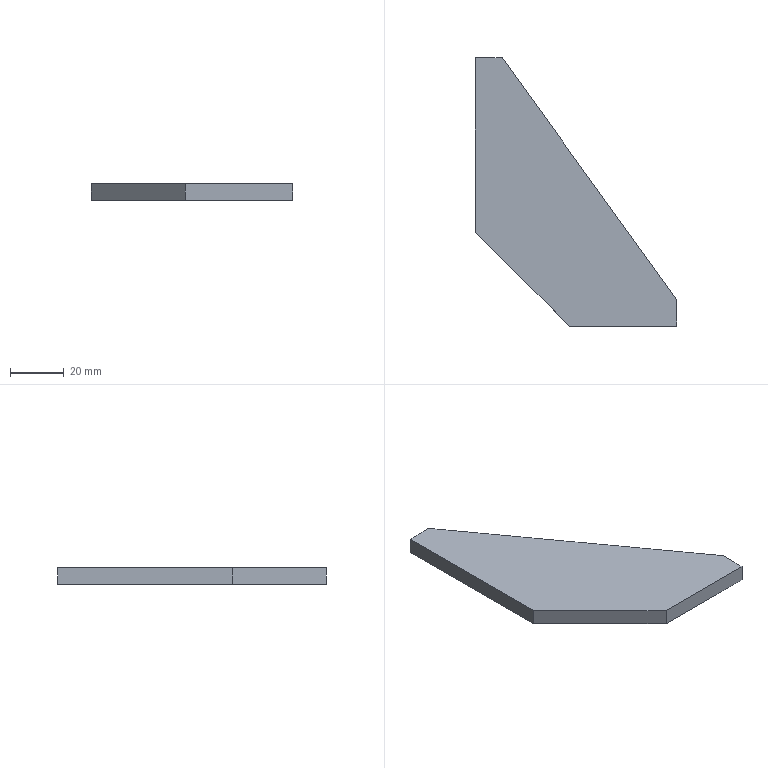Part | SolidWorks | features Chamfer 1, Extrusion 1 | 1 solid | 8 faces | box 75 x 100 x 6 mm | volume 23775 mm3 | plane 8
STEP:
#1=CARTESIAN_POINT('',(10.,100.,-3.));
#2=VERTEX_POINT('',#1);
#3=CARTESIAN_POINT('',(0.,100.,-3.));
#4=VERTEX_POINT('',#3);
#5=CARTESIAN_POINT('',(10.,100.,-3.));
#6=DIRECTION('',(-1.,0.,0.));
#7=VECTOR('',#6,1000.);
#8=LINE('',#5,#7);
#9=EDGE_CURVE('',#2,#4,#8,.T.);
#10=ORIENTED_EDGE('',*,*,#9,.T.);
#11=CARTESIAN_POINT('',(0.,100.,3.));
#12=VERTEX_POINT('',#11);
#13=CARTESIAN_POINT('',(0.,100.,3.));
#14=DIRECTION('',(0.,0.,-1.));
#15=VECTOR('',#14,1000.);
#16=LINE('',#13,#15);
#17=EDGE_CURVE('',#12,#4,#16,.T.);
#18=ORIENTED_EDGE('',*,*,#17,.F.);
#19=CARTESIAN_POINT('',(10.,100.,3.));
#20=VERTEX_POINT('',#19);
#21=CARTESIAN_POINT('',(10.,100.,3.));
#22=DIRECTION('',(-1.,0.,0.));
#23=VECTOR('',#22,1000.);
#24=LINE('',#21,#23);
#25=EDGE_CURVE('',#20,#12,#24,.T.);
#26=ORIENTED_EDGE('',*,*,#25,.F.);
#27=CARTESIAN_POINT('',(10.,100.,3.));
#28=DIRECTION('',(0.,0.,-1.));
#29=VECTOR('',#28,1000.);
#30=LINE('',#27,#29);
#31=EDGE_CURVE('',#20,#2,#30,.T.);
#32=ORIENTED_EDGE('',*,*,#31,.T.);
#33=EDGE_LOOP('',(#10,#18,#26,#32));
#34=FACE_OUTER_BOUND('',#33,.T.);
#35=CARTESIAN_POINT('',(10.,100.,3.));
#36=DIRECTION('',(0.,-1.,0.));
#37=DIRECTION('',(0.,0.,-1.));
#38=AXIS2_PLACEMENT_3D('',#35,#36,#37);
#39=PLANE('',#38);
#40=ADVANCED_FACE('',(#34),#39,.F.);
#41=CARTESIAN_POINT('',(0.,35.,-3.));
#42=VERTEX_POINT('',#41);
#43=CARTESIAN_POINT('',(0.,100.,-3.));
#44=DIRECTION('',(0.,-1.,0.));
#45=VECTOR('',#44,1000.);
#46=LINE('',#43,#45);
#47=EDGE_CURVE('',#4,#42,#46,.T.);
#48=ORIENTED_EDGE('',*,*,#47,.T.);
#49=CARTESIAN_POINT('',(0.,35.,3.));
#50=VERTEX_POINT('',#49);
#51=CARTESIAN_POINT('',(0.,35.,3.));
#52=DIRECTION('',(0.,0.,1.));
#53=VECTOR('',#52,1000.);
#54=LINE('',#51,#53);
#55=EDGE_CURVE('',#42,#50,#54,.T.);
#56=ORIENTED_EDGE('',*,*,#55,.T.);
#57=CARTESIAN_POINT('',(0.,100.,3.));
#58=DIRECTION('',(0.,-1.,0.));
#59=VECTOR('',#58,1000.);
#60=LINE('',#57,#59);
#61=EDGE_CURVE('',#12,#50,#60,.T.);
#62=ORIENTED_EDGE('',*,*,#61,.F.);
#63=ORIENTED_EDGE('',*,*,#17,.T.);
#64=EDGE_LOOP('',(#48,#56,#62,#63));
#65=FACE_OUTER_BOUND('',#64,.T.);
#66=CARTESIAN_POINT('',(0.,100.,3.));
#67=DIRECTION('',(1.,0.,0.));
#68=DIRECTION('',(0.,1.,0.));
#69=AXIS2_PLACEMENT_3D('',#66,#67,#68);
#70=PLANE('',#69);
#71=ADVANCED_FACE('',(#65),#70,.F.);
#72=CARTESIAN_POINT('',(35.,0.,3.));
#73=VERTEX_POINT('',#72);
#74=CARTESIAN_POINT('',(75.,0.,3.));
#75=VERTEX_POINT('',#74);
#76=CARTESIAN_POINT('',(0.,0.,3.));
#77=DIRECTION('',(1.,0.,0.));
#78=VECTOR('',#77,1000.);
#79=LINE('',#76,#78);
#80=EDGE_CURVE('',#73,#75,#79,.T.);
#81=ORIENTED_EDGE('',*,*,#80,.F.);
#82=CARTESIAN_POINT('',(35.,0.,-3.));
#83=VERTEX_POINT('',#82);
#84=CARTESIAN_POINT('',(35.,0.,3.));
#85=DIRECTION('',(0.,0.,-1.));
#86=VECTOR('',#85,1000.);
#87=LINE('',#84,#86);
#88=EDGE_CURVE('',#73,#83,#87,.T.);
#89=ORIENTED_EDGE('',*,*,#88,.T.);
#90=CARTESIAN_POINT('',(75.,0.,-3.));
#91=VERTEX_POINT('',#90);
#92=CARTESIAN_POINT('',(0.,0.,-3.));
#93=DIRECTION('',(1.,0.,0.));
#94=VECTOR('',#93,1000.);
#95=LINE('',#92,#94);
#96=EDGE_CURVE('',#83,#91,#95,.T.);
#97=ORIENTED_EDGE('',*,*,#96,.T.);
#98=CARTESIAN_POINT('',(75.,0.,3.));
#99=DIRECTION('',(0.,0.,-1.));
#100=VECTOR('',#99,1000.);
#101=LINE('',#98,#100);
#102=EDGE_CURVE('',#75,#91,#101,.T.);
#103=ORIENTED_EDGE('',*,*,#102,.F.);
#104=EDGE_LOOP('',(#81,#89,#97,#103));
#105=FACE_OUTER_BOUND('',#104,.T.);
#106=CARTESIAN_POINT('',(0.,0.,3.));
#107=DIRECTION('',(0.,1.,0.));
#108=DIRECTION('',(0.,0.,1.));
#109=AXIS2_PLACEMENT_3D('',#106,#107,#108);
#110=PLANE('',#109);
#111=ADVANCED_FACE('',(#105),#110,.F.);
#112=CARTESIAN_POINT('',(75.,10.,-3.));
#113=VERTEX_POINT('',#112);
#114=CARTESIAN_POINT('',(75.,0.,-3.));
#115=DIRECTION('',(0.,1.,0.));
#116=VECTOR('',#115,1000.);
#117=LINE('',#114,#116);
#118=EDGE_CURVE('',#91,#113,#117,.T.);
#119=ORIENTED_EDGE('',*,*,#118,.T.);
#120=CARTESIAN_POINT('',(75.,10.,3.));
#121=VERTEX_POINT('',#120);
#122=CARTESIAN_POINT('',(75.,10.,3.));
#123=DIRECTION('',(0.,0.,-1.));
#124=VECTOR('',#123,1000.);
#125=LINE('',#122,#124);
#126=EDGE_CURVE('',#121,#113,#125,.T.);
#127=ORIENTED_EDGE('',*,*,#126,.F.);
#128=CARTESIAN_POINT('',(75.,0.,3.));
#129=DIRECTION('',(0.,1.,0.));
#130=VECTOR('',#129,1000.);
#131=LINE('',#128,#130);
#132=EDGE_CURVE('',#75,#121,#131,.T.);
#133=ORIENTED_EDGE('',*,*,#132,.F.);
#134=ORIENTED_EDGE('',*,*,#102,.T.);
#135=EDGE_LOOP('',(#119,#127,#133,#134));
#136=FACE_OUTER_BOUND('',#135,.T.);
#137=CARTESIAN_POINT('',(75.,0.,3.));
#138=DIRECTION('',(-1.,0.,0.));
#139=DIRECTION('',(0.,0.,1.));
#140=AXIS2_PLACEMENT_3D('',#137,#138,#139);
#141=PLANE('',#140);
#142=ADVANCED_FACE('',(#136),#141,.F.);
#143=CARTESIAN_POINT('',(75.,10.,-3.));
#144=DIRECTION('',(-0.5855,0.8107,0.));
#145=VECTOR('',#144,1000.);
#146=LINE('',#143,#145);
#147=EDGE_CURVE('',#113,#2,#146,.T.);
#148=ORIENTED_EDGE('',*,*,#147,.T.);
#149=ORIENTED_EDGE('',*,*,#31,.F.);
#150=CARTESIAN_POINT('',(75.,10.,3.));
#151=DIRECTION('',(-0.5855,0.8107,0.));
#152=VECTOR('',#151,1000.);
#153=LINE('',#150,#152);
#154=EDGE_CURVE('',#121,#20,#153,.T.);
#155=ORIENTED_EDGE('',*,*,#154,.F.);
#156=ORIENTED_EDGE('',*,*,#126,.T.);
#157=EDGE_LOOP('',(#148,#149,#155,#156));
#158=FACE_OUTER_BOUND('',#157,.T.);
#159=CARTESIAN_POINT('',(75.,10.,3.));
#160=DIRECTION('',(-0.8107,-0.5855,0.));
#161=DIRECTION('',(0.5855,-0.8107,0.));
#162=AXIS2_PLACEMENT_3D('',#159,#160,#161);
#163=PLANE('',#162);
#164=ADVANCED_FACE('',(#158),#163,.F.);
#165=ORIENTED_EDGE('',*,*,#61,.T.);
#166=CARTESIAN_POINT('',(17.5,17.5,3.));
#167=DIRECTION('',(0.7071,-0.7071,0.));
#168=VECTOR('',#167,1000.);
#169=LINE('',#166,#168);
#170=EDGE_CURVE('',#50,#73,#169,.T.);
#171=ORIENTED_EDGE('',*,*,#170,.T.);
#172=ORIENTED_EDGE('',*,*,#80,.T.);
#173=ORIENTED_EDGE('',*,*,#132,.T.);
#174=ORIENTED_EDGE('',*,*,#154,.T.);
#175=ORIENTED_EDGE('',*,*,#25,.T.);
#176=EDGE_LOOP('',(#165,#171,#172,#173,#174,#175));
#177=FACE_OUTER_BOUND('',#176,.T.);
#178=CARTESIAN_POINT('',(0.,0.,3.));
#179=DIRECTION('',(0.,0.,1.));
#180=DIRECTION('',(1.,0.,0.));
#181=AXIS2_PLACEMENT_3D('',#178,#179,#180);
#182=PLANE('',#181);
#183=ADVANCED_FACE('',(#177),#182,.T.);
#184=ORIENTED_EDGE('',*,*,#96,.F.);
#185=CARTESIAN_POINT('',(35.,0.,-3.));
#186=DIRECTION('',(-0.7071,0.7071,0.));
#187=VECTOR('',#186,1000.);
#188=LINE('',#185,#187);
#189=EDGE_CURVE('',#83,#42,#188,.T.);
#190=ORIENTED_EDGE('',*,*,#189,.T.);
#191=ORIENTED_EDGE('',*,*,#47,.F.);
#192=ORIENTED_EDGE('',*,*,#9,.F.);
#193=ORIENTED_EDGE('',*,*,#147,.F.);
#194=ORIENTED_EDGE('',*,*,#118,.F.);
#195=EDGE_LOOP('',(#184,#190,#191,#192,#193,#194));
#196=FACE_OUTER_BOUND('',#195,.T.);
#197=CARTESIAN_POINT('',(0.,0.,-3.));
#198=DIRECTION('',(0.,0.,1.));
#199=DIRECTION('',(1.,0.,0.));
#200=AXIS2_PLACEMENT_3D('',#197,#198,#199);
#201=PLANE('',#200);
#202=ADVANCED_FACE('',(#196),#201,.F.);
#203=ORIENTED_EDGE('',*,*,#170,.F.);
#204=ORIENTED_EDGE('',*,*,#55,.F.);
#205=ORIENTED_EDGE('',*,*,#189,.F.);
#206=ORIENTED_EDGE('',*,*,#88,.F.);
#207=EDGE_LOOP('',(#203,#204,#205,#206));
#208=FACE_OUTER_BOUND('',#207,.T.);
#209=CARTESIAN_POINT('',(35.,0.,3.));
#210=DIRECTION('',(0.7071,0.7071,0.));
#211=DIRECTION('',(0.,0.,-1.));
#212=AXIS2_PLACEMENT_3D('',#209,#210,#211);
#213=PLANE('',#212);
#214=ADVANCED_FACE('',(#208),#213,.F.);
#215=CLOSED_SHELL('',(#40,#71,#111,#142,#164,#183,#202,#214));
#216=MANIFOLD_SOLID_BREP('',#215);
#217=CARTESIAN_POINT('',(0.,0.,0.));
#218=DIRECTION('',(0.,0.,1.));
#219=DIRECTION('',(1.,0.,0.));
#220=AXIS2_PLACEMENT_3D('',#217,#218,#219);
#221=(LENGTH_UNIT()NAMED_UNIT(*)SI_UNIT(.MILLI.,.METRE.));
#222=UNCERTAINTY_MEASURE_WITH_UNIT(LENGTH_MEASURE(0.00001),#221,'','');
#223=(NAMED_UNIT(*)PLANE_ANGLE_UNIT()SI_UNIT($,.RADIAN.));
#224=(NAMED_UNIT(*)SI_UNIT($,.STERADIAN.)SOLID_ANGLE_UNIT());
#225=(GEOMETRIC_REPRESENTATION_CONTEXT(3)GLOBAL_UNCERTAINTY_ASSIGNED_CONTEXT((#222))GLOBAL_UNIT_ASSIGNED_CONTEXT((#221,#223,#224))REPRESENTATION_CONTEXT('',''));
#226=ADVANCED_BREP_SHAPE_REPRESENTATION('',(#216,#220),#225);